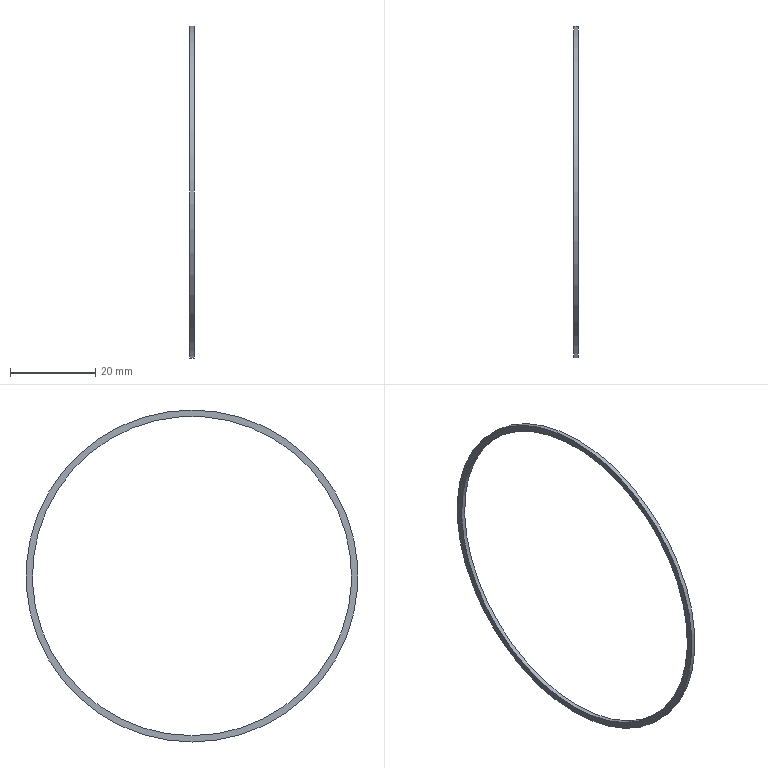Part | STEP file | Outer seal of clamping device | 1 solid | 4 faces | box 1 x 78 x 78 mm | volume 360.498 mm3 | plane 2 | cylinder 2 | commonest cylinder face diameters 75 x1 78 x1
STEP:
#1=CARTESIAN_POINT('',(0.,0.,-39.));
#2=VERTEX_POINT('',#1);
#3=CARTESIAN_POINT('',(0.,0.,0.));
#4=DIRECTION('',(1.,0.,0.));
#5=DIRECTION('',(0.,0.,-1.));
#6=AXIS2_PLACEMENT_3D('',#3,#4,#5);
#7=CIRCLE('',#6,39.);
#8=EDGE_CURVE('',#2,#2,#7,.T.);
#9=ORIENTED_EDGE('',*,*,#8,.F.);
#10=EDGE_LOOP('',(#9));
#11=FACE_BOUND('',#10,.T.);
#12=CARTESIAN_POINT('',(0.,0.,-37.5));
#13=VERTEX_POINT('',#12);
#14=CARTESIAN_POINT('',(0.,0.,0.));
#15=DIRECTION('',(1.,0.,0.));
#16=DIRECTION('',(0.,0.,-1.));
#17=AXIS2_PLACEMENT_3D('',#14,#15,#16);
#18=CIRCLE('',#17,37.5);
#19=EDGE_CURVE('',#13,#13,#18,.T.);
#20=ORIENTED_EDGE('',*,*,#19,.T.);
#21=EDGE_LOOP('',(#20));
#22=FACE_BOUND('',#21,.T.);
#23=CARTESIAN_POINT('',(0.,0.,0.));
#24=DIRECTION('',(1.,0.,0.));
#25=DIRECTION('',(0.,0.,-1.));
#26=AXIS2_PLACEMENT_3D('',#23,#24,#25);
#27=PLANE('',#26);
#28=ADVANCED_FACE('',(#11,#22),#27,.F.);
#29=CARTESIAN_POINT('',(1.,0.,-39.));
#30=VERTEX_POINT('',#29);
#31=CARTESIAN_POINT('',(1.,0.,0.));
#32=DIRECTION('',(1.,0.,0.));
#33=DIRECTION('',(0.,0.,-1.));
#34=AXIS2_PLACEMENT_3D('',#31,#32,#33);
#35=CIRCLE('',#34,39.);
#36=EDGE_CURVE('',#30,#30,#35,.T.);
#37=ORIENTED_EDGE('',*,*,#36,.T.);
#38=EDGE_LOOP('',(#37));
#39=FACE_BOUND('',#38,.T.);
#40=CARTESIAN_POINT('',(1.,0.,-37.5));
#41=VERTEX_POINT('',#40);
#42=CARTESIAN_POINT('',(1.,0.,0.));
#43=DIRECTION('',(1.,0.,0.));
#44=DIRECTION('',(0.,0.,-1.));
#45=AXIS2_PLACEMENT_3D('',#42,#43,#44);
#46=CIRCLE('',#45,37.5);
#47=EDGE_CURVE('',#41,#41,#46,.F.);
#48=ORIENTED_EDGE('',*,*,#47,.T.);
#49=EDGE_LOOP('',(#48));
#50=FACE_BOUND('',#49,.T.);
#51=CARTESIAN_POINT('',(1.,0.,0.));
#52=DIRECTION('',(1.,0.,0.));
#53=DIRECTION('',(0.,0.,-1.));
#54=AXIS2_PLACEMENT_3D('',#51,#52,#53);
#55=PLANE('',#54);
#56=ADVANCED_FACE('',(#39,#50),#55,.T.);
#57=ORIENTED_EDGE('',*,*,#47,.F.);
#58=EDGE_LOOP('',(#57));
#59=FACE_OUTER_BOUND('',#58,.T.);
#60=ORIENTED_EDGE('',*,*,#19,.F.);
#61=EDGE_LOOP('',(#60));
#62=FACE_OUTER_BOUND('',#61,.T.);
#63=CARTESIAN_POINT('',(0.,0.,0.));
#64=DIRECTION('',(1.,0.,0.));
#65=DIRECTION('',(0.,0.,-1.));
#66=AXIS2_PLACEMENT_3D('',#63,#64,#65);
#67=CYLINDRICAL_SURFACE('',#66,37.5);
#68=ADVANCED_FACE('',(#59,#62),#67,.F.);
#69=ORIENTED_EDGE('',*,*,#36,.F.);
#70=EDGE_LOOP('',(#69));
#71=FACE_OUTER_BOUND('',#70,.T.);
#72=ORIENTED_EDGE('',*,*,#8,.T.);
#73=EDGE_LOOP('',(#72));
#74=FACE_OUTER_BOUND('',#73,.T.);
#75=CARTESIAN_POINT('',(0.,0.,0.));
#76=DIRECTION('',(1.,0.,0.));
#77=DIRECTION('',(0.,0.,-1.));
#78=AXIS2_PLACEMENT_3D('',#75,#76,#77);
#79=CYLINDRICAL_SURFACE('',#78,39.);
#80=ADVANCED_FACE('',(#71,#74),#79,.T.);
#81=CLOSED_SHELL('',(#28,#56,#68,#80));
#82=MANIFOLD_SOLID_BREP('',#81);
#83=(LENGTH_UNIT()NAMED_UNIT(*)SI_UNIT(.MILLI.,.METRE.));
#84=UNCERTAINTY_MEASURE_WITH_UNIT(LENGTH_MEASURE(0.00001),#83,'','');
#85=(NAMED_UNIT(*)PLANE_ANGLE_UNIT()SI_UNIT($,.RADIAN.));
#86=(NAMED_UNIT(*)SI_UNIT($,.STERADIAN.)SOLID_ANGLE_UNIT());
#87=(GEOMETRIC_REPRESENTATION_CONTEXT(3)GLOBAL_UNCERTAINTY_ASSIGNED_CONTEXT((#84))GLOBAL_UNIT_ASSIGNED_CONTEXT((#83,#85,#86))REPRESENTATION_CONTEXT('',''));
#88=ADVANCED_BREP_SHAPE_REPRESENTATION('',(#82),#87);